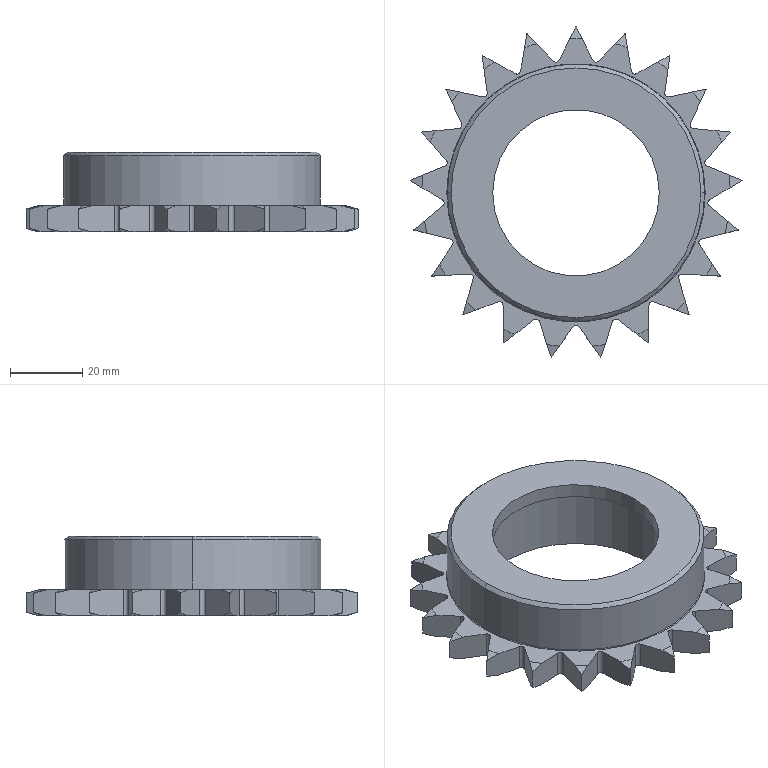Part | STEP file | PN_0022_SP40B21-N-25 | 1 solid | 167 faces | box 91.743 x 91.486 x 22 mm | volume 50734 mm3 | plane 46 | cone 44 | torus 44 | cylinder 33 | commonest cylinder face diameters 2 x27 46 x2 52 x2 71 x2